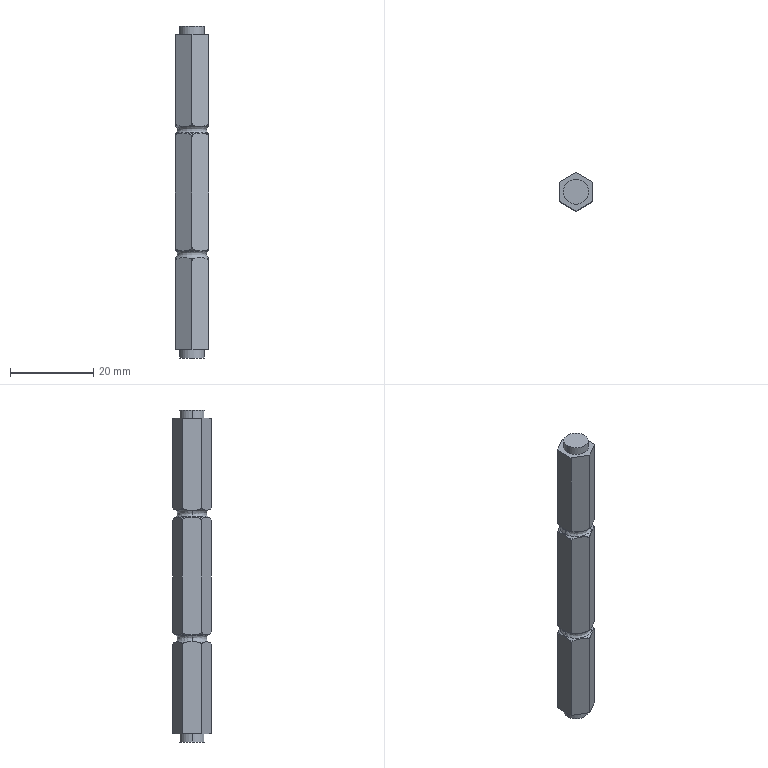Part | STEP file | 1 solid | 62 faces | box 8 x 9.238 x 80 mm | volume 4280 mm3 | spline 28 | plane 22 | cone 8 | cylinder 4 | commonest cylinder face diameters 6 x4